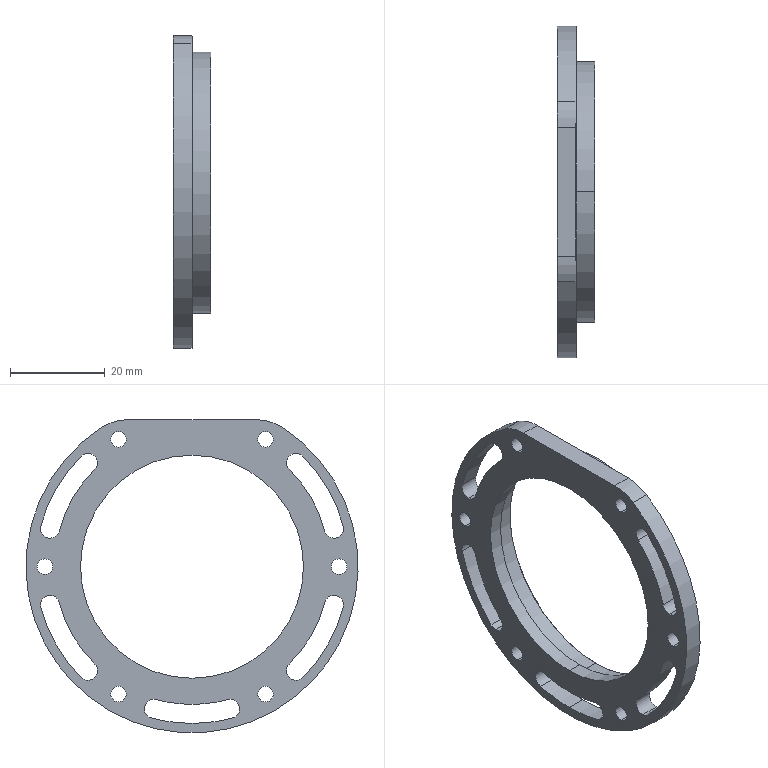Part | SolidWorks | features ICE 2, Chamfer 1, Fillet 1, HoleWzd 1, Revolution 1 | 1 solid | 54 faces | box 8 x 70 x 66 mm | volume 7364 mm3 | cylinder 47 | plane 5 | cone 2 | commonest cylinder face diameters 4 x14 3.3 x12 58 x6 66 x6 20 x2 47 x2